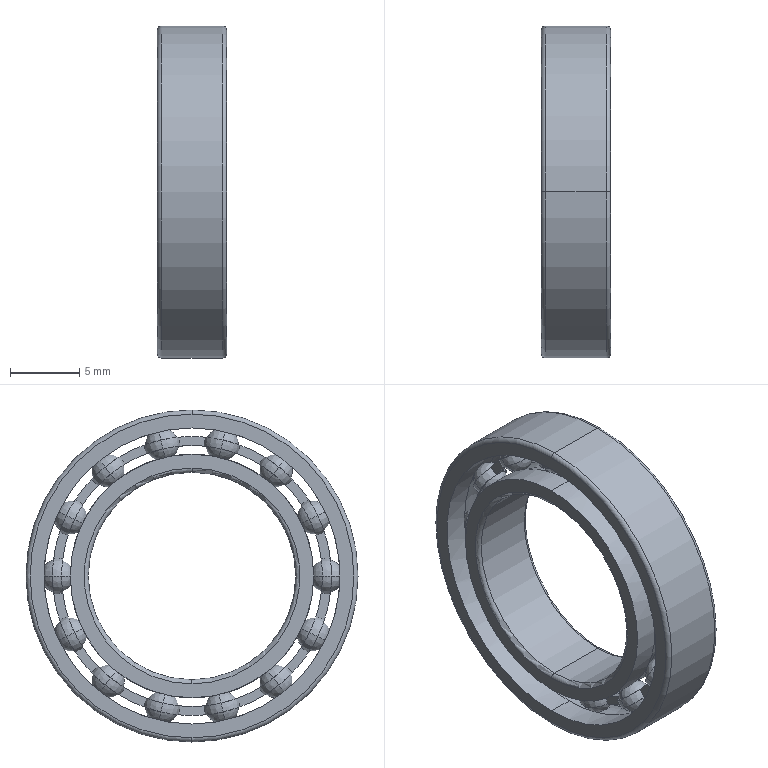Part | SolidWorks | features Revolution 5, CirPattern 2, RevCut 2 | 1 solid | 213 faces | box 5 x 24 x 24 mm | volume 880.809 mm3 | sphere 112 | torus 53 | plane 32 | cylinder 16 | commonest cylinder face diameters 17.6 x4 21.4 x4 15 x2 18.845 x2 20.155 x2 24 x2